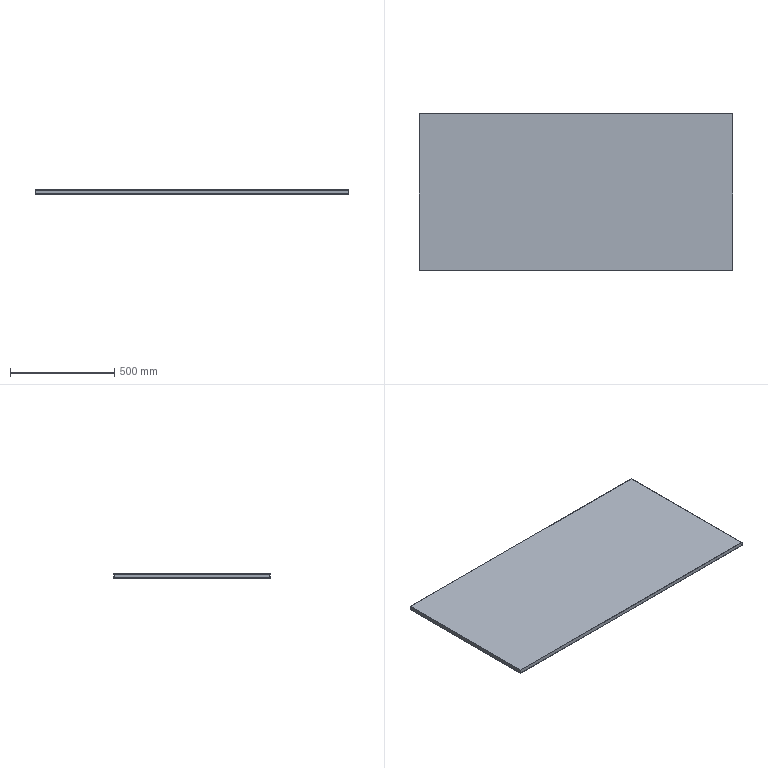Part | STEP file | 1 solid | 16 faces | box 1500 x 750 x 20 mm | volume 1901997 mm3 | plane 16
STEP:
#1=CARTESIAN_POINT('',(0.,0.,0.));
#2=DIRECTION('',(0.,0.,1.));
#3=DIRECTION('',(1.,0.,0.));
#4=AXIS2_PLACEMENT_3D('',#1,#2,#3);
#5=CARTESIAN_POINT('',(750.,-375.,20.));
#6=VERTEX_POINT('',#5);
#7=CARTESIAN_POINT('',(750.,375.,20.));
#8=VERTEX_POINT('',#7);
#9=CARTESIAN_POINT('',(750.,-375.,20.));
#10=DIRECTION('',(0.,1.,0.));
#11=VECTOR('',#10,1.);
#12=LINE('',#9,#11);
#13=CARTESIAN_POINT('',(750.,-375.,20.));
#14=DIRECTION('',(0.,0.,1.));
#15=DIRECTION('',(1.,0.,0.));
#16=AXIS2_PLACEMENT_3D('',#13,#14,#15);
#17=PLANE('',#16);
#18=CARTESIAN_POINT('',(0.,0.));
#19=DIRECTION('',(0.,1.));
#20=VECTOR('',#19,1.);
#21=LINE('',#18,#20);
#22=(GEOMETRIC_REPRESENTATION_CONTEXT(2)PARAMETRIC_REPRESENTATION_CONTEXT()REPRESENTATION_CONTEXT('',''));
#23=DEFINITIONAL_REPRESENTATION('',(#21),#22);
#24=PCURVE('',#17,#23);
#25=CARTESIAN_POINT('',(750.,375.,20.));
#26=DIRECTION('',(-1.,0.,0.));
#27=DIRECTION('',(0.,-1.,0.));
#28=AXIS2_PLACEMENT_3D('',#25,#26,#27);
#29=PLANE('',#28);
#30=CARTESIAN_POINT('',(750.,0.));
#31=DIRECTION('',(-1.,0.));
#32=VECTOR('',#31,1.);
#33=LINE('',#30,#32);
#34=(GEOMETRIC_REPRESENTATION_CONTEXT(2)PARAMETRIC_REPRESENTATION_CONTEXT()REPRESENTATION_CONTEXT('',''));
#35=DEFINITIONAL_REPRESENTATION('',(#33),#34);
#36=PCURVE('',#29,#35);
#37=SURFACE_CURVE('',#12,(#24,#36),.PCURVE_S1.);
#38=EDGE_CURVE('',#6,#8,#37,.T.);
#39=ORIENTED_EDGE('',*,*,#38,.T.);
#40=CARTESIAN_POINT('',(-750.,375.,20.));
#41=VERTEX_POINT('',#40);
#42=CARTESIAN_POINT('',(750.,375.,20.));
#43=DIRECTION('',(-1.,0.,0.));
#44=VECTOR('',#43,1.);
#45=LINE('',#42,#44);
#46=CARTESIAN_POINT('',(0.,750.));
#47=DIRECTION('',(-1.,0.));
#48=VECTOR('',#47,1.);
#49=LINE('',#46,#48);
#50=(GEOMETRIC_REPRESENTATION_CONTEXT(2)PARAMETRIC_REPRESENTATION_CONTEXT()REPRESENTATION_CONTEXT('',''));
#51=DEFINITIONAL_REPRESENTATION('',(#49),#50);
#52=PCURVE('',#17,#51);
#53=CARTESIAN_POINT('',(-750.,375.,20.));
#54=DIRECTION('',(0.,-1.,0.));
#55=DIRECTION('',(0.,0.,-1.));
#56=AXIS2_PLACEMENT_3D('',#53,#54,#55);
#57=PLANE('',#56);
#58=CARTESIAN_POINT('',(0.,1500.));
#59=DIRECTION('',(0.,-1.));
#60=VECTOR('',#59,1.);
#61=LINE('',#58,#60);
#62=(GEOMETRIC_REPRESENTATION_CONTEXT(2)PARAMETRIC_REPRESENTATION_CONTEXT()REPRESENTATION_CONTEXT('',''));
#63=DEFINITIONAL_REPRESENTATION('',(#61),#62);
#64=PCURVE('',#57,#63);
#65=SURFACE_CURVE('',#45,(#52,#64),.PCURVE_S1.);
#66=EDGE_CURVE('',#8,#41,#65,.T.);
#67=ORIENTED_EDGE('',*,*,#66,.T.);
#68=CARTESIAN_POINT('',(-750.,-375.,20.));
#69=VERTEX_POINT('',#68);
#70=CARTESIAN_POINT('',(-750.,-375.,20.));
#71=DIRECTION('',(0.,-1.,0.));
#72=VECTOR('',#71,1.);
#73=LINE('',#70,#72);
#74=CARTESIAN_POINT('',(-1500.,0.));
#75=DIRECTION('',(0.,-1.));
#76=VECTOR('',#75,1.);
#77=LINE('',#74,#76);
#78=(GEOMETRIC_REPRESENTATION_CONTEXT(2)PARAMETRIC_REPRESENTATION_CONTEXT()REPRESENTATION_CONTEXT('',''));
#79=DEFINITIONAL_REPRESENTATION('',(#77),#78);
#80=PCURVE('',#17,#79);
#81=CARTESIAN_POINT('',(-750.,375.,20.));
#82=DIRECTION('',(1.,0.,0.));
#83=DIRECTION('',(0.,1.,0.));
#84=AXIS2_PLACEMENT_3D('',#81,#82,#83);
#85=PLANE('',#84);
#86=CARTESIAN_POINT('',(-750.,0.));
#87=DIRECTION('',(-1.,0.));
#88=VECTOR('',#87,1.);
#89=LINE('',#86,#88);
#90=(GEOMETRIC_REPRESENTATION_CONTEXT(2)PARAMETRIC_REPRESENTATION_CONTEXT()REPRESENTATION_CONTEXT('',''));
#91=DEFINITIONAL_REPRESENTATION('',(#89),#90);
#92=PCURVE('',#85,#91);
#93=SURFACE_CURVE('',#73,(#80,#92),.PCURVE_S1.);
#94=EDGE_CURVE('',#41,#69,#93,.T.);
#95=ORIENTED_EDGE('',*,*,#94,.T.);
#96=CARTESIAN_POINT('',(750.,-375.,20.));
#97=DIRECTION('',(1.,0.,0.));
#98=VECTOR('',#97,1.);
#99=LINE('',#96,#98);
#100=CARTESIAN_POINT('',(0.,0.));
#101=DIRECTION('',(1.,0.));
#102=VECTOR('',#101,1.);
#103=LINE('',#100,#102);
#104=(GEOMETRIC_REPRESENTATION_CONTEXT(2)PARAMETRIC_REPRESENTATION_CONTEXT()REPRESENTATION_CONTEXT('',''));
#105=DEFINITIONAL_REPRESENTATION('',(#103),#104);
#106=PCURVE('',#17,#105);
#107=CARTESIAN_POINT('',(-750.,-375.,20.));
#108=DIRECTION('',(0.,1.,0.));
#109=DIRECTION('',(0.,0.,1.));
#110=AXIS2_PLACEMENT_3D('',#107,#108,#109);
#111=PLANE('',#110);
#112=CARTESIAN_POINT('',(0.,1500.));
#113=DIRECTION('',(0.,1.));
#114=VECTOR('',#113,1.);
#115=LINE('',#112,#114);
#116=(GEOMETRIC_REPRESENTATION_CONTEXT(2)PARAMETRIC_REPRESENTATION_CONTEXT()REPRESENTATION_CONTEXT('',''));
#117=DEFINITIONAL_REPRESENTATION('',(#115),#116);
#118=PCURVE('',#111,#117);
#119=SURFACE_CURVE('',#99,(#106,#118),.PCURVE_S1.);
#120=EDGE_CURVE('',#69,#6,#119,.T.);
#121=ORIENTED_EDGE('',*,*,#120,.T.);
#122=EDGE_LOOP('',(#39,#67,#95,#121));
#123=FACE_BOUND('',#122,.T.);
#124=ADVANCED_FACE('',(#123),#17,.T.);
#125=ORIENTED_EDGE('',*,*,#66,.F.);
#126=CARTESIAN_POINT('',(750.,375.,0.));
#127=VERTEX_POINT('',#126);
#128=CARTESIAN_POINT('',(750.,375.,20.));
#129=DIRECTION('',(0.,0.,1.));
#130=VECTOR('',#129,1.);
#131=LINE('',#128,#130);
#132=CARTESIAN_POINT('',(0.,1500.));
#133=DIRECTION('',(-1.,0.));
#134=VECTOR('',#133,1.);
#135=LINE('',#132,#134);
#136=(GEOMETRIC_REPRESENTATION_CONTEXT(2)PARAMETRIC_REPRESENTATION_CONTEXT()REPRESENTATION_CONTEXT('',''));
#137=DEFINITIONAL_REPRESENTATION('',(#135),#136);
#138=PCURVE('',#57,#137);
#139=CARTESIAN_POINT('',(0.,0.));
#140=DIRECTION('',(0.,1.));
#141=VECTOR('',#140,1.);
#142=LINE('',#139,#141);
#143=(GEOMETRIC_REPRESENTATION_CONTEXT(2)PARAMETRIC_REPRESENTATION_CONTEXT()REPRESENTATION_CONTEXT('',''));
#144=DEFINITIONAL_REPRESENTATION('',(#142),#143);
#145=PCURVE('',#29,#144);
#146=SURFACE_CURVE('',#131,(#138,#145),.PCURVE_S1.);
#147=EDGE_CURVE('',#127,#8,#146,.T.);
#148=ORIENTED_EDGE('',*,*,#147,.F.);
#149=CARTESIAN_POINT('',(-750.,375.,0.));
#150=VERTEX_POINT('',#149);
#151=CARTESIAN_POINT('',(-750.,375.,0.));
#152=DIRECTION('',(1.,0.,0.));
#153=VECTOR('',#152,1.);
#154=LINE('',#151,#153);
#155=CARTESIAN_POINT('',(20.,0.));
#156=DIRECTION('',(0.,1.));
#157=VECTOR('',#156,1.);
#158=LINE('',#155,#157);
#159=(GEOMETRIC_REPRESENTATION_CONTEXT(2)PARAMETRIC_REPRESENTATION_CONTEXT()REPRESENTATION_CONTEXT('',''));
#160=DEFINITIONAL_REPRESENTATION('',(#158),#159);
#161=PCURVE('',#57,#160);
#162=CARTESIAN_POINT('',(750.,-375.,0.));
#163=DIRECTION('',(0.,0.,1.));
#164=DIRECTION('',(1.,0.,0.));
#165=AXIS2_PLACEMENT_3D('',#162,#163,#164);
#166=PLANE('',#165);
#167=CARTESIAN_POINT('',(-1500.,750.));
#168=DIRECTION('',(1.,0.));
#169=VECTOR('',#168,1.);
#170=LINE('',#167,#169);
#171=(GEOMETRIC_REPRESENTATION_CONTEXT(2)PARAMETRIC_REPRESENTATION_CONTEXT()REPRESENTATION_CONTEXT('',''));
#172=DEFINITIONAL_REPRESENTATION('',(#170),#171);
#173=PCURVE('',#166,#172);
#174=SURFACE_CURVE('',#154,(#161,#173),.PCURVE_S1.);
#175=EDGE_CURVE('',#150,#127,#174,.T.);
#176=ORIENTED_EDGE('',*,*,#175,.F.);
#177=CARTESIAN_POINT('',(-750.,375.,20.));
#178=DIRECTION('',(0.,0.,-1.));
#179=VECTOR('',#178,1.);
#180=LINE('',#177,#179);
#181=CARTESIAN_POINT('',(0.,0.));
#182=DIRECTION('',(1.,0.));
#183=VECTOR('',#182,1.);
#184=LINE('',#181,#183);
#185=(GEOMETRIC_REPRESENTATION_CONTEXT(2)PARAMETRIC_REPRESENTATION_CONTEXT()REPRESENTATION_CONTEXT('',''));
#186=DEFINITIONAL_REPRESENTATION('',(#184),#185);
#187=PCURVE('',#57,#186);
#188=CARTESIAN_POINT('',(0.,0.));
#189=DIRECTION('',(0.,-1.));
#190=VECTOR('',#189,1.);
#191=LINE('',#188,#190);
#192=(GEOMETRIC_REPRESENTATION_CONTEXT(2)PARAMETRIC_REPRESENTATION_CONTEXT()REPRESENTATION_CONTEXT('',''));
#193=DEFINITIONAL_REPRESENTATION('',(#191),#192);
#194=PCURVE('',#85,#193);
#195=SURFACE_CURVE('',#180,(#187,#194),.PCURVE_S1.);
#196=EDGE_CURVE('',#41,#150,#195,.T.);
#197=ORIENTED_EDGE('',*,*,#196,.F.);
#198=EDGE_LOOP('',(#125,#148,#176,#197));
#199=FACE_BOUND('',#198,.T.);
#200=ADVANCED_FACE('',(#199),#57,.F.);
#201=ORIENTED_EDGE('',*,*,#38,.F.);
#202=CARTESIAN_POINT('',(750.,-375.,0.));
#203=VERTEX_POINT('',#202);
#204=CARTESIAN_POINT('',(750.,-375.,20.));
#205=DIRECTION('',(0.,0.,1.));
#206=VECTOR('',#205,1.);
#207=LINE('',#204,#206);
#208=CARTESIAN_POINT('',(750.,0.));
#209=DIRECTION('',(0.,1.));
#210=VECTOR('',#209,1.);
#211=LINE('',#208,#210);
#212=(GEOMETRIC_REPRESENTATION_CONTEXT(2)PARAMETRIC_REPRESENTATION_CONTEXT()REPRESENTATION_CONTEXT('',''));
#213=DEFINITIONAL_REPRESENTATION('',(#211),#212);
#214=PCURVE('',#29,#213);
#215=CARTESIAN_POINT('',(0.,1500.));
#216=DIRECTION('',(1.,0.));
#217=VECTOR('',#216,1.);
#218=LINE('',#215,#217);
#219=(GEOMETRIC_REPRESENTATION_CONTEXT(2)PARAMETRIC_REPRESENTATION_CONTEXT()REPRESENTATION_CONTEXT('',''));
#220=DEFINITIONAL_REPRESENTATION('',(#218),#219);
#221=PCURVE('',#111,#220);
#222=SURFACE_CURVE('',#207,(#214,#221),.PCURVE_S1.);
#223=EDGE_CURVE('',#203,#6,#222,.T.);
#224=ORIENTED_EDGE('',*,*,#223,.F.);
#225=CARTESIAN_POINT('',(750.,375.,0.));
#226=DIRECTION('',(0.,-1.,0.));
#227=VECTOR('',#226,1.);
#228=LINE('',#225,#227);
#229=CARTESIAN_POINT('',(0.,-20.));
#230=DIRECTION('',(1.,0.));
#231=VECTOR('',#230,1.);
#232=LINE('',#229,#231);
#233=(GEOMETRIC_REPRESENTATION_CONTEXT(2)PARAMETRIC_REPRESENTATION_CONTEXT()REPRESENTATION_CONTEXT('',''));
#234=DEFINITIONAL_REPRESENTATION('',(#232),#233);
#235=PCURVE('',#29,#234);
#236=CARTESIAN_POINT('',(0.,750.));
#237=DIRECTION('',(0.,-1.));
#238=VECTOR('',#237,1.);
#239=LINE('',#236,#238);
#240=(GEOMETRIC_REPRESENTATION_CONTEXT(2)PARAMETRIC_REPRESENTATION_CONTEXT()REPRESENTATION_CONTEXT('',''));
#241=DEFINITIONAL_REPRESENTATION('',(#239),#240);
#242=PCURVE('',#166,#241);
#243=SURFACE_CURVE('',#228,(#235,#242),.PCURVE_S1.);
#244=EDGE_CURVE('',#127,#203,#243,.T.);
#245=ORIENTED_EDGE('',*,*,#244,.F.);
#246=ORIENTED_EDGE('',*,*,#147,.T.);
#247=EDGE_LOOP('',(#201,#224,#245,#246));
#248=FACE_BOUND('',#247,.T.);
#249=ADVANCED_FACE('',(#248),#29,.F.);
#250=ORIENTED_EDGE('',*,*,#120,.F.);
#251=CARTESIAN_POINT('',(-750.,-375.,0.));
#252=VERTEX_POINT('',#251);
#253=CARTESIAN_POINT('',(-750.,-375.,20.));
#254=DIRECTION('',(0.,0.,1.));
#255=VECTOR('',#254,1.);
#256=LINE('',#253,#255);
#257=CARTESIAN_POINT('',(0.,0.));
#258=DIRECTION('',(1.,0.));
#259=VECTOR('',#258,1.);
#260=LINE('',#257,#259);
#261=(GEOMETRIC_REPRESENTATION_CONTEXT(2)PARAMETRIC_REPRESENTATION_CONTEXT()REPRESENTATION_CONTEXT('',''));
#262=DEFINITIONAL_REPRESENTATION('',(#260),#261);
#263=PCURVE('',#111,#262);
#264=CARTESIAN_POINT('',(-750.,0.));
#265=DIRECTION('',(0.,1.));
#266=VECTOR('',#265,1.);
#267=LINE('',#264,#266);
#268=(GEOMETRIC_REPRESENTATION_CONTEXT(2)PARAMETRIC_REPRESENTATION_CONTEXT()REPRESENTATION_CONTEXT('',''));
#269=DEFINITIONAL_REPRESENTATION('',(#267),#268);
#270=PCURVE('',#85,#269);
#271=SURFACE_CURVE('',#256,(#263,#270),.PCURVE_S1.);
#272=EDGE_CURVE('',#252,#69,#271,.T.);
#273=ORIENTED_EDGE('',*,*,#272,.F.);
#274=CARTESIAN_POINT('',(-750.,-375.,0.));
#275=DIRECTION('',(-1.,0.,0.));
#276=VECTOR('',#275,1.);
#277=LINE('',#274,#276);
#278=CARTESIAN_POINT('',(-20.,0.));
#279=DIRECTION('',(0.,-1.));
#280=VECTOR('',#279,1.);
#281=LINE('',#278,#280);
#282=(GEOMETRIC_REPRESENTATION_CONTEXT(2)PARAMETRIC_REPRESENTATION_CONTEXT()REPRESENTATION_CONTEXT('',''));
#283=DEFINITIONAL_REPRESENTATION('',(#281),#282);
#284=PCURVE('',#111,#283);
#285=CARTESIAN_POINT('',(-1500.,0.));
#286=DIRECTION('',(-1.,0.));
#287=VECTOR('',#286,1.);
#288=LINE('',#285,#287);
#289=(GEOMETRIC_REPRESENTATION_CONTEXT(2)PARAMETRIC_REPRESENTATION_CONTEXT()REPRESENTATION_CONTEXT('',''));
#290=DEFINITIONAL_REPRESENTATION('',(#288),#289);
#291=PCURVE('',#166,#290);
#292=SURFACE_CURVE('',#277,(#284,#291),.PCURVE_S1.);
#293=EDGE_CURVE('',#203,#252,#292,.T.);
#294=ORIENTED_EDGE('',*,*,#293,.F.);
#295=ORIENTED_EDGE('',*,*,#223,.T.);
#296=EDGE_LOOP('',(#250,#273,#294,#295));
#297=FACE_BOUND('',#296,.T.);
#298=ADVANCED_FACE('',(#297),#111,.F.);
#299=ORIENTED_EDGE('',*,*,#94,.F.);
#300=ORIENTED_EDGE('',*,*,#196,.T.);
#301=CARTESIAN_POINT('',(-750.,375.,0.));
#302=DIRECTION('',(0.,1.,0.));
#303=VECTOR('',#302,1.);
#304=LINE('',#301,#303);
#305=CARTESIAN_POINT('',(0.,-20.));
#306=DIRECTION('',(1.,0.));
#307=VECTOR('',#306,1.);
#308=LINE('',#305,#307);
#309=(GEOMETRIC_REPRESENTATION_CONTEXT(2)PARAMETRIC_REPRESENTATION_CONTEXT()REPRESENTATION_CONTEXT('',''));
#310=DEFINITIONAL_REPRESENTATION('',(#308),#309);
#311=PCURVE('',#85,#310);
#312=CARTESIAN_POINT('',(-1500.,750.));
#313=DIRECTION('',(0.,1.));
#314=VECTOR('',#313,1.);
#315=LINE('',#312,#314);
#316=(GEOMETRIC_REPRESENTATION_CONTEXT(2)PARAMETRIC_REPRESENTATION_CONTEXT()REPRESENTATION_CONTEXT('',''));
#317=DEFINITIONAL_REPRESENTATION('',(#315),#316);
#318=PCURVE('',#166,#317);
#319=SURFACE_CURVE('',#304,(#311,#318),.PCURVE_S1.);
#320=EDGE_CURVE('',#252,#150,#319,.T.);
#321=ORIENTED_EDGE('',*,*,#320,.F.);
#322=ORIENTED_EDGE('',*,*,#272,.T.);
#323=EDGE_LOOP('',(#299,#300,#321,#322));
#324=FACE_BOUND('',#323,.T.);
#325=ADVANCED_FACE('',(#324),#85,.F.);
#326=CARTESIAN_POINT('',(735.,360.,0.));
#327=VERTEX_POINT('',#326);
#328=CARTESIAN_POINT('',(735.,-360.,0.));
#329=VERTEX_POINT('',#328);
#330=CARTESIAN_POINT('',(735.,-375.,0.));
#331=DIRECTION('',(0.,-1.,0.));
#332=VECTOR('',#331,1.);
#333=LINE('',#330,#332);
#334=CARTESIAN_POINT('',(-15.,0.));
#335=DIRECTION('',(0.,-1.));
#336=VECTOR('',#335,1.);
#337=LINE('',#334,#336);
#338=(GEOMETRIC_REPRESENTATION_CONTEXT(2)PARAMETRIC_REPRESENTATION_CONTEXT()REPRESENTATION_CONTEXT('',''));
#339=DEFINITIONAL_REPRESENTATION('',(#337),#338);
#340=PCURVE('',#166,#339);
#341=CARTESIAN_POINT('',(735.,360.,1.5));
#342=DIRECTION('',(1.,0.,0.));
#343=DIRECTION('',(0.,0.,-1.));
#344=AXIS2_PLACEMENT_3D('',#341,#342,#343);
#345=PLANE('',#344);
#346=CARTESIAN_POINT('',(1.5,-735.));
#347=DIRECTION('',(0.,-1.));
#348=VECTOR('',#347,1.);
#349=LINE('',#346,#348);
#350=(GEOMETRIC_REPRESENTATION_CONTEXT(2)PARAMETRIC_REPRESENTATION_CONTEXT()REPRESENTATION_CONTEXT('',''));
#351=DEFINITIONAL_REPRESENTATION('',(#349),#350);
#352=PCURVE('',#345,#351);
#353=SURFACE_CURVE('',#333,(#340,#352),.PCURVE_S1.);
#354=EDGE_CURVE('',#327,#329,#353,.T.);
#355=ORIENTED_EDGE('',*,*,#354,.F.);
#356=CARTESIAN_POINT('',(-735.,360.,0.));
#357=VERTEX_POINT('',#356);
#358=CARTESIAN_POINT('',(750.,360.,0.));
#359=DIRECTION('',(1.,0.,0.));
#360=VECTOR('',#359,1.);
#361=LINE('',#358,#360);
#362=CARTESIAN_POINT('',(0.,735.));
#363=DIRECTION('',(1.,0.));
#364=VECTOR('',#363,1.);
#365=LINE('',#362,#364);
#366=(GEOMETRIC_REPRESENTATION_CONTEXT(2)PARAMETRIC_REPRESENTATION_CONTEXT()REPRESENTATION_CONTEXT('',''));
#367=DEFINITIONAL_REPRESENTATION('',(#365),#366);
#368=PCURVE('',#166,#367);
#369=CARTESIAN_POINT('',(735.,360.,1.5));
#370=DIRECTION('',(0.,1.,0.));
#371=DIRECTION('',(0.,0.,1.));
#372=AXIS2_PLACEMENT_3D('',#369,#370,#371);
#373=PLANE('',#372);
#374=CARTESIAN_POINT('',(-1.5,15.));
#375=DIRECTION('',(0.,1.));
#376=VECTOR('',#375,1.);
#377=LINE('',#374,#376);
#378=(GEOMETRIC_REPRESENTATION_CONTEXT(2)PARAMETRIC_REPRESENTATION_CONTEXT()REPRESENTATION_CONTEXT('',''));
#379=DEFINITIONAL_REPRESENTATION('',(#377),#378);
#380=PCURVE('',#373,#379);
#381=SURFACE_CURVE('',#361,(#368,#380),.PCURVE_S1.);
#382=EDGE_CURVE('',#357,#327,#381,.T.);
#383=ORIENTED_EDGE('',*,*,#382,.F.);
#384=CARTESIAN_POINT('',(-735.,-360.,0.));
#385=VERTEX_POINT('',#384);
#386=CARTESIAN_POINT('',(-735.,-375.,0.));
#387=DIRECTION('',(0.,1.,0.));
#388=VECTOR('',#387,1.);
#389=LINE('',#386,#388);
#390=CARTESIAN_POINT('',(-1485.,0.));
#391=DIRECTION('',(0.,1.));
#392=VECTOR('',#391,1.);
#393=LINE('',#390,#392);
#394=(GEOMETRIC_REPRESENTATION_CONTEXT(2)PARAMETRIC_REPRESENTATION_CONTEXT()REPRESENTATION_CONTEXT('',''));
#395=DEFINITIONAL_REPRESENTATION('',(#393),#394);
#396=PCURVE('',#166,#395);
#397=CARTESIAN_POINT('',(-735.,360.,1.5));
#398=DIRECTION('',(-1.,0.,0.));
#399=DIRECTION('',(0.,0.,1.));
#400=AXIS2_PLACEMENT_3D('',#397,#398,#399);
#401=PLANE('',#400);
#402=CARTESIAN_POINT('',(-1.5,-735.));
#403=DIRECTION('',(0.,1.));
#404=VECTOR('',#403,1.);
#405=LINE('',#402,#404);
#406=(GEOMETRIC_REPRESENTATION_CONTEXT(2)PARAMETRIC_REPRESENTATION_CONTEXT()REPRESENTATION_CONTEXT('',''));
#407=DEFINITIONAL_REPRESENTATION('',(#405),#406);
#408=PCURVE('',#401,#407);
#409=SURFACE_CURVE('',#389,(#396,#408),.PCURVE_S1.);
#410=EDGE_CURVE('',#385,#357,#409,.T.);
#411=ORIENTED_EDGE('',*,*,#410,.F.);
#412=CARTESIAN_POINT('',(750.,-360.,0.));
#413=DIRECTION('',(-1.,0.,0.));
#414=VECTOR('',#413,1.);
#415=LINE('',#412,#414);
#416=CARTESIAN_POINT('',(0.,15.));
#417=DIRECTION('',(-1.,0.));
#418=VECTOR('',#417,1.);
#419=LINE('',#416,#418);
#420=(GEOMETRIC_REPRESENTATION_CONTEXT(2)PARAMETRIC_REPRESENTATION_CONTEXT()REPRESENTATION_CONTEXT('',''));
#421=DEFINITIONAL_REPRESENTATION('',(#419),#420);
#422=PCURVE('',#166,#421);
#423=CARTESIAN_POINT('',(735.,-360.,1.5));
#424=DIRECTION('',(0.,-1.,0.));
#425=DIRECTION('',(0.,0.,-1.));
#426=AXIS2_PLACEMENT_3D('',#423,#424,#425);
#427=PLANE('',#426);
#428=CARTESIAN_POINT('',(1.5,15.));
#429=DIRECTION('',(0.,-1.));
#430=VECTOR('',#429,1.);
#431=LINE('',#428,#430);
#432=(GEOMETRIC_REPRESENTATION_CONTEXT(2)PARAMETRIC_REPRESENTATION_CONTEXT()REPRESENTATION_CONTEXT('',''));
#433=DEFINITIONAL_REPRESENTATION('',(#431),#432);
#434=PCURVE('',#427,#433);
#435=SURFACE_CURVE('',#415,(#422,#434),.PCURVE_S1.);
#436=EDGE_CURVE('',#329,#385,#435,.T.);
#437=ORIENTED_EDGE('',*,*,#436,.F.);
#438=EDGE_LOOP('',(#355,#383,#411,#437));
#439=FACE_BOUND('',#438,.T.);
#440=ORIENTED_EDGE('',*,*,#320,.T.);
#441=ORIENTED_EDGE('',*,*,#175,.T.);
#442=ORIENTED_EDGE('',*,*,#244,.T.);
#443=ORIENTED_EDGE('',*,*,#293,.T.);
#444=EDGE_LOOP('',(#440,#441,#442,#443));
#445=FACE_BOUND('',#444,.T.);
#446=ADVANCED_FACE('',(#439,#445),#166,.F.);
#447=CARTESIAN_POINT('',(735.,-360.,1.5));
#448=VERTEX_POINT('',#447);
#449=CARTESIAN_POINT('',(-735.,-360.,1.5));
#450=VERTEX_POINT('',#449);
#451=CARTESIAN_POINT('',(735.,-360.,1.5));
#452=DIRECTION('',(-1.,0.,0.));
#453=VECTOR('',#452,1.);
#454=LINE('',#451,#453);
#455=CARTESIAN_POINT('',(0.,0.));
#456=DIRECTION('',(0.,-1.));
#457=VECTOR('',#456,1.);
#458=LINE('',#455,#457);
#459=(GEOMETRIC_REPRESENTATION_CONTEXT(2)PARAMETRIC_REPRESENTATION_CONTEXT()REPRESENTATION_CONTEXT('',''));
#460=DEFINITIONAL_REPRESENTATION('',(#458),#459);
#461=PCURVE('',#427,#460);
#462=CARTESIAN_POINT('',(-750.,-375.,1.5));
#463=DIRECTION('',(0.,0.,-1.));
#464=DIRECTION('',(-1.,0.,0.));
#465=AXIS2_PLACEMENT_3D('',#462,#463,#464);
#466=PLANE('',#465);
#467=CARTESIAN_POINT('',(-1485.,15.));
#468=DIRECTION('',(1.,0.));
#469=VECTOR('',#468,1.);
#470=LINE('',#467,#469);
#471=(GEOMETRIC_REPRESENTATION_CONTEXT(2)PARAMETRIC_REPRESENTATION_CONTEXT()REPRESENTATION_CONTEXT('',''));
#472=DEFINITIONAL_REPRESENTATION('',(#470),#471);
#473=PCURVE('',#466,#472);
#474=SURFACE_CURVE('',#454,(#461,#473),.PCURVE_S1.);
#475=EDGE_CURVE('',#448,#450,#474,.T.);
#476=ORIENTED_EDGE('',*,*,#475,.F.);
#477=CARTESIAN_POINT('',(735.,-360.,1.5));
#478=DIRECTION('',(0.,0.,1.));
#479=VECTOR('',#478,1.);
#480=LINE('',#477,#479);
#481=CARTESIAN_POINT('',(0.,0.));
#482=DIRECTION('',(-1.,0.));
#483=VECTOR('',#482,1.);
#484=LINE('',#481,#483);
#485=(GEOMETRIC_REPRESENTATION_CONTEXT(2)PARAMETRIC_REPRESENTATION_CONTEXT()REPRESENTATION_CONTEXT('',''));
#486=DEFINITIONAL_REPRESENTATION('',(#484),#485);
#487=PCURVE('',#427,#486);
#488=CARTESIAN_POINT('',(0.,-720.));
#489=DIRECTION('',(-1.,0.));
#490=VECTOR('',#489,1.);
#491=LINE('',#488,#490);
#492=(GEOMETRIC_REPRESENTATION_CONTEXT(2)PARAMETRIC_REPRESENTATION_CONTEXT()REPRESENTATION_CONTEXT('',''));
#493=DEFINITIONAL_REPRESENTATION('',(#491),#492);
#494=PCURVE('',#345,#493);
#495=SURFACE_CURVE('',#480,(#487,#494),.PCURVE_S1.);
#496=EDGE_CURVE('',#329,#448,#495,.T.);
#497=ORIENTED_EDGE('',*,*,#496,.F.);
#498=ORIENTED_EDGE('',*,*,#436,.T.);
#499=CARTESIAN_POINT('',(-735.,-360.,1.5));
#500=DIRECTION('',(0.,0.,-1.));
#501=VECTOR('',#500,1.);
#502=LINE('',#499,#501);
#503=CARTESIAN_POINT('',(0.,-1470.));
#504=DIRECTION('',(1.,0.));
#505=VECTOR('',#504,1.);
#506=LINE('',#503,#505);
#507=(GEOMETRIC_REPRESENTATION_CONTEXT(2)PARAMETRIC_REPRESENTATION_CONTEXT()REPRESENTATION_CONTEXT('',''));
#508=DEFINITIONAL_REPRESENTATION('',(#506),#507);
#509=PCURVE('',#427,#508);
#510=CARTESIAN_POINT('',(0.,-720.));
#511=DIRECTION('',(-1.,0.));
#512=VECTOR('',#511,1.);
#513=LINE('',#510,#512);
#514=(GEOMETRIC_REPRESENTATION_CONTEXT(2)PARAMETRIC_REPRESENTATION_CONTEXT()REPRESENTATION_CONTEXT('',''));
#515=DEFINITIONAL_REPRESENTATION('',(#513),#514);
#516=PCURVE('',#401,#515);
#517=SURFACE_CURVE('',#502,(#509,#516),.PCURVE_S1.);
#518=EDGE_CURVE('',#450,#385,#517,.T.);
#519=ORIENTED_EDGE('',*,*,#518,.F.);
#520=EDGE_LOOP('',(#476,#497,#498,#519));
#521=FACE_BOUND('',#520,.T.);
#522=ADVANCED_FACE('',(#521),#427,.F.);
#523=CARTESIAN_POINT('',(735.,360.,1.5));
#524=VERTEX_POINT('',#523);
#525=CARTESIAN_POINT('',(735.,360.,1.5));
#526=DIRECTION('',(0.,-1.,0.));
#527=VECTOR('',#526,1.);
#528=LINE('',#525,#527);
#529=CARTESIAN_POINT('',(0.,0.));
#530=DIRECTION('',(0.,-1.));
#531=VECTOR('',#530,1.);
#532=LINE('',#529,#531);
#533=(GEOMETRIC_REPRESENTATION_CONTEXT(2)PARAMETRIC_REPRESENTATION_CONTEXT()REPRESENTATION_CONTEXT('',''));
#534=DEFINITIONAL_REPRESENTATION('',(#532),#533);
#535=PCURVE('',#345,#534);
#536=CARTESIAN_POINT('',(-1485.,735.));
#537=DIRECTION('',(0.,-1.));
#538=VECTOR('',#537,1.);
#539=LINE('',#536,#538);
#540=(GEOMETRIC_REPRESENTATION_CONTEXT(2)PARAMETRIC_REPRESENTATION_CONTEXT()REPRESENTATION_CONTEXT('',''));
#541=DEFINITIONAL_REPRESENTATION('',(#539),#540);
#542=PCURVE('',#466,#541);
#543=SURFACE_CURVE('',#528,(#535,#542),.PCURVE_S1.);
#544=EDGE_CURVE('',#524,#448,#543,.T.);
#545=ORIENTED_EDGE('',*,*,#544,.F.);
#546=CARTESIAN_POINT('',(735.,360.,1.5));
#547=DIRECTION('',(0.,0.,1.));
#548=VECTOR('',#547,1.);
#549=LINE('',#546,#548);
#550=CARTESIAN_POINT('',(0.,0.));
#551=DIRECTION('',(-1.,0.));
#552=VECTOR('',#551,1.);
#553=LINE('',#550,#552);
#554=(GEOMETRIC_REPRESENTATION_CONTEXT(2)PARAMETRIC_REPRESENTATION_CONTEXT()REPRESENTATION_CONTEXT('',''));
#555=DEFINITIONAL_REPRESENTATION('',(#553),#554);
#556=PCURVE('',#345,#555);
#557=CARTESIAN_POINT('',(0.,0.));
#558=DIRECTION('',(1.,0.));
#559=VECTOR('',#558,1.);
#560=LINE('',#557,#559);
#561=(GEOMETRIC_REPRESENTATION_CONTEXT(2)PARAMETRIC_REPRESENTATION_CONTEXT()REPRESENTATION_CONTEXT('',''));
#562=DEFINITIONAL_REPRESENTATION('',(#560),#561);
#563=PCURVE('',#373,#562);
#564=SURFACE_CURVE('',#549,(#556,#563),.PCURVE_S1.);
#565=EDGE_CURVE('',#327,#524,#564,.T.);
#566=ORIENTED_EDGE('',*,*,#565,.F.);
#567=ORIENTED_EDGE('',*,*,#354,.T.);
#568=ORIENTED_EDGE('',*,*,#496,.T.);
#569=EDGE_LOOP('',(#545,#566,#567,#568));
#570=FACE_BOUND('',#569,.T.);
#571=ADVANCED_FACE('',(#570),#345,.F.);
#572=CARTESIAN_POINT('',(-735.,360.,1.5));
#573=VERTEX_POINT('',#572);
#574=CARTESIAN_POINT('',(735.,360.,1.5));
#575=DIRECTION('',(1.,0.,0.));
#576=VECTOR('',#575,1.);
#577=LINE('',#574,#576);
#578=CARTESIAN_POINT('',(0.,0.));
#579=DIRECTION('',(0.,1.));
#580=VECTOR('',#579,1.);
#581=LINE('',#578,#580);
#582=(GEOMETRIC_REPRESENTATION_CONTEXT(2)PARAMETRIC_REPRESENTATION_CONTEXT()REPRESENTATION_CONTEXT('',''));
#583=DEFINITIONAL_REPRESENTATION('',(#581),#582);
#584=PCURVE('',#373,#583);
#585=CARTESIAN_POINT('',(-1485.,735.));
#586=DIRECTION('',(-1.,0.));
#587=VECTOR('',#586,1.);
#588=LINE('',#585,#587);
#589=(GEOMETRIC_REPRESENTATION_CONTEXT(2)PARAMETRIC_REPRESENTATION_CONTEXT()REPRESENTATION_CONTEXT('',''));
#590=DEFINITIONAL_REPRESENTATION('',(#588),#589);
#591=PCURVE('',#466,#590);
#592=SURFACE_CURVE('',#577,(#584,#591),.PCURVE_S1.);
#593=EDGE_CURVE('',#573,#524,#592,.T.);
#594=ORIENTED_EDGE('',*,*,#593,.F.);
#595=CARTESIAN_POINT('',(-735.,360.,1.5));
#596=DIRECTION('',(0.,0.,1.));
#597=VECTOR('',#596,1.);
#598=LINE('',#595,#597);
#599=CARTESIAN_POINT('',(0.,-1470.));
#600=DIRECTION('',(1.,0.));
#601=VECTOR('',#600,1.);
#602=LINE('',#599,#601);
#603=(GEOMETRIC_REPRESENTATION_CONTEXT(2)PARAMETRIC_REPRESENTATION_CONTEXT()REPRESENTATION_CONTEXT('',''));
#604=DEFINITIONAL_REPRESENTATION('',(#602),#603);
#605=PCURVE('',#373,#604);
#606=CARTESIAN_POINT('',(0.,0.));
#607=DIRECTION('',(1.,0.));
#608=VECTOR('',#607,1.);
#609=LINE('',#606,#608);
#610=(GEOMETRIC_REPRESENTATION_CONTEXT(2)PARAMETRIC_REPRESENTATION_CONTEXT()REPRESENTATION_CONTEXT('',''));
#611=DEFINITIONAL_REPRESENTATION('',(#609),#610);
#612=PCURVE('',#401,#611);
#613=SURFACE_CURVE('',#598,(#605,#612),.PCURVE_S1.);
#614=EDGE_CURVE('',#357,#573,#613,.T.);
#615=ORIENTED_EDGE('',*,*,#614,.F.);
#616=ORIENTED_EDGE('',*,*,#382,.T.);
#617=ORIENTED_EDGE('',*,*,#565,.T.);
#618=EDGE_LOOP('',(#594,#615,#616,#617));
#619=FACE_BOUND('',#618,.T.);
#620=ADVANCED_FACE('',(#619),#373,.F.);
#621=CARTESIAN_POINT('',(-735.,360.,1.5));
#622=DIRECTION('',(0.,1.,0.));
#623=VECTOR('',#622,1.);
#624=LINE('',#621,#623);
#625=CARTESIAN_POINT('',(0.,0.));
#626=DIRECTION('',(0.,1.));
#627=VECTOR('',#626,1.);
#628=LINE('',#625,#627);
#629=(GEOMETRIC_REPRESENTATION_CONTEXT(2)PARAMETRIC_REPRESENTATION_CONTEXT()REPRESENTATION_CONTEXT('',''));
#630=DEFINITIONAL_REPRESENTATION('',(#628),#629);
#631=PCURVE('',#401,#630);
#632=CARTESIAN_POINT('',(-15.,735.));
#633=DIRECTION('',(0.,1.));
#634=VECTOR('',#633,1.);
#635=LINE('',#632,#634);
#636=(GEOMETRIC_REPRESENTATION_CONTEXT(2)PARAMETRIC_REPRESENTATION_CONTEXT()REPRESENTATION_CONTEXT('',''));
#637=DEFINITIONAL_REPRESENTATION('',(#635),#636);
#638=PCURVE('',#466,#637);
#639=SURFACE_CURVE('',#624,(#631,#638),.PCURVE_S1.);
#640=EDGE_CURVE('',#450,#573,#639,.T.);
#641=ORIENTED_EDGE('',*,*,#640,.F.);
#642=ORIENTED_EDGE('',*,*,#518,.T.);
#643=ORIENTED_EDGE('',*,*,#410,.T.);
#644=ORIENTED_EDGE('',*,*,#614,.T.);
#645=EDGE_LOOP('',(#641,#642,#643,#644));
#646=FACE_BOUND('',#645,.T.);
#647=ADVANCED_FACE('',(#646),#401,.F.);
#648=ORIENTED_EDGE('',*,*,#593,.T.);
#649=ORIENTED_EDGE('',*,*,#544,.T.);
#650=ORIENTED_EDGE('',*,*,#475,.T.);
#651=ORIENTED_EDGE('',*,*,#640,.T.);
#652=EDGE_LOOP('',(#648,#649,#650,#651));
#653=FACE_BOUND('',#652,.T.);
#654=CARTESIAN_POINT('',(-748.5,-373.5,1.5));
#655=VERTEX_POINT('',#654);
#656=CARTESIAN_POINT('',(-748.5,373.5,1.5));
#657=VERTEX_POINT('',#656);
#658=CARTESIAN_POINT('',(-748.5,-375.,1.5));
#659=DIRECTION('',(0.,1.,0.));
#660=VECTOR('',#659,1.);
#661=LINE('',#658,#660);
#662=CARTESIAN_POINT('',(-1.5,0.));
#663=DIRECTION('',(0.,1.));
#664=VECTOR('',#663,1.);
#665=LINE('',#662,#664);
#666=(GEOMETRIC_REPRESENTATION_CONTEXT(2)PARAMETRIC_REPRESENTATION_CONTEXT()REPRESENTATION_CONTEXT('',''));
#667=DEFINITIONAL_REPRESENTATION('',(#665),#666);
#668=PCURVE('',#466,#667);
#669=CARTESIAN_POINT('',(-748.5,375.,20.));
#670=DIRECTION('',(1.,0.,0.));
#671=DIRECTION('',(0.,1.,0.));
#672=AXIS2_PLACEMENT_3D('',#669,#670,#671);
#673=PLANE('',#672);
#674=CARTESIAN_POINT('',(-750.,-18.5));
#675=DIRECTION('',(1.,0.));
#676=VECTOR('',#675,1.);
#677=LINE('',#674,#676);
#678=(GEOMETRIC_REPRESENTATION_CONTEXT(2)PARAMETRIC_REPRESENTATION_CONTEXT()REPRESENTATION_CONTEXT('',''));
#679=DEFINITIONAL_REPRESENTATION('',(#677),#678);
#680=PCURVE('',#673,#679);
#681=SURFACE_CURVE('',#661,(#668,#680),.PCURVE_S1.);
#682=EDGE_CURVE('',#655,#657,#681,.T.);
#683=ORIENTED_EDGE('',*,*,#682,.F.);
#684=CARTESIAN_POINT('',(748.5,-373.5,1.5));
#685=VERTEX_POINT('',#684);
#686=CARTESIAN_POINT('',(-750.,-373.5,1.5));
#687=DIRECTION('',(-1.,0.,0.));
#688=VECTOR('',#687,1.);
#689=LINE('',#686,#688);
#690=CARTESIAN_POINT('',(0.,1.5));
#691=DIRECTION('',(1.,0.));
#692=VECTOR('',#691,1.);
#693=LINE('',#690,#692);
#694=(GEOMETRIC_REPRESENTATION_CONTEXT(2)PARAMETRIC_REPRESENTATION_CONTEXT()REPRESENTATION_CONTEXT('',''));
#695=DEFINITIONAL_REPRESENTATION('',(#693),#694);
#696=PCURVE('',#466,#695);
#697=CARTESIAN_POINT('',(-750.,-373.5,20.));
#698=DIRECTION('',(0.,1.,0.));
#699=DIRECTION('',(0.,0.,1.));
#700=AXIS2_PLACEMENT_3D('',#697,#698,#699);
#701=PLANE('',#700);
#702=CARTESIAN_POINT('',(-18.5,0.));
#703=DIRECTION('',(0.,-1.));
#704=VECTOR('',#703,1.);
#705=LINE('',#702,#704);
#706=(GEOMETRIC_REPRESENTATION_CONTEXT(2)PARAMETRIC_REPRESENTATION_CONTEXT()REPRESENTATION_CONTEXT('',''));
#707=DEFINITIONAL_REPRESENTATION('',(#705),#706);
#708=PCURVE('',#701,#707);
#709=SURFACE_CURVE('',#689,(#696,#708),.PCURVE_S1.);
#710=EDGE_CURVE('',#685,#655,#709,.T.);
#711=ORIENTED_EDGE('',*,*,#710,.F.);
#712=CARTESIAN_POINT('',(748.5,373.5,1.5));
#713=VERTEX_POINT('',#712);
#714=CARTESIAN_POINT('',(748.5,-375.,1.5));
#715=DIRECTION('',(0.,-1.,0.));
#716=VECTOR('',#715,1.);
#717=LINE('',#714,#716);
#718=CARTESIAN_POINT('',(-1498.5,0.));
#719=DIRECTION('',(0.,-1.));
#720=VECTOR('',#719,1.);
#721=LINE('',#718,#720);
#722=(GEOMETRIC_REPRESENTATION_CONTEXT(2)PARAMETRIC_REPRESENTATION_CONTEXT()REPRESENTATION_CONTEXT('',''));
#723=DEFINITIONAL_REPRESENTATION('',(#721),#722);
#724=PCURVE('',#466,#723);
#725=CARTESIAN_POINT('',(748.5,375.,20.));
#726=DIRECTION('',(-1.,0.,0.));
#727=DIRECTION('',(0.,-1.,0.));
#728=AXIS2_PLACEMENT_3D('',#725,#726,#727);
#729=PLANE('',#728);
#730=CARTESIAN_POINT('',(750.,-18.5));
#731=DIRECTION('',(1.,0.));
#732=VECTOR('',#731,1.);
#733=LINE('',#730,#732);
#734=(GEOMETRIC_REPRESENTATION_CONTEXT(2)PARAMETRIC_REPRESENTATION_CONTEXT()REPRESENTATION_CONTEXT('',''));
#735=DEFINITIONAL_REPRESENTATION('',(#733),#734);
#736=PCURVE('',#729,#735);
#737=SURFACE_CURVE('',#717,(#724,#736),.PCURVE_S1.);
#738=EDGE_CURVE('',#713,#685,#737,.T.);
#739=ORIENTED_EDGE('',*,*,#738,.F.);
#740=CARTESIAN_POINT('',(-750.,373.5,1.5));
#741=DIRECTION('',(1.,0.,0.));
#742=VECTOR('',#741,1.);
#743=LINE('',#740,#742);
#744=CARTESIAN_POINT('',(0.,748.5));
#745=DIRECTION('',(-1.,0.));
#746=VECTOR('',#745,1.);
#747=LINE('',#744,#746);
#748=(GEOMETRIC_REPRESENTATION_CONTEXT(2)PARAMETRIC_REPRESENTATION_CONTEXT()REPRESENTATION_CONTEXT('',''));
#749=DEFINITIONAL_REPRESENTATION('',(#747),#748);
#750=PCURVE('',#466,#749);
#751=CARTESIAN_POINT('',(-750.,373.5,20.));
#752=DIRECTION('',(0.,-1.,0.));
#753=DIRECTION('',(0.,0.,-1.));
#754=AXIS2_PLACEMENT_3D('',#751,#752,#753);
#755=PLANE('',#754);
#756=CARTESIAN_POINT('',(18.5,0.));
#757=DIRECTION('',(0.,1.));
#758=VECTOR('',#757,1.);
#759=LINE('',#756,#758);
#760=(GEOMETRIC_REPRESENTATION_CONTEXT(2)PARAMETRIC_REPRESENTATION_CONTEXT()REPRESENTATION_CONTEXT('',''));
#761=DEFINITIONAL_REPRESENTATION('',(#759),#760);
#762=PCURVE('',#755,#761);
#763=SURFACE_CURVE('',#743,(#750,#762),.PCURVE_S1.);
#764=EDGE_CURVE('',#657,#713,#763,.T.);
#765=ORIENTED_EDGE('',*,*,#764,.F.);
#766=EDGE_LOOP('',(#683,#711,#739,#765));
#767=FACE_BOUND('',#766,.T.);
#768=ADVANCED_FACE('',(#653,#767),#466,.F.);
#769=CARTESIAN_POINT('',(-748.5,373.5,18.5));
#770=VERTEX_POINT('',#769);
#771=CARTESIAN_POINT('',(-748.5,373.5,20.));
#772=DIRECTION('',(0.,0.,-1.));
#773=VECTOR('',#772,1.);
#774=LINE('',#771,#773);
#775=CARTESIAN_POINT('',(0.,1.5));
#776=DIRECTION('',(1.,0.));
#777=VECTOR('',#776,1.);
#778=LINE('',#775,#777);
#779=(GEOMETRIC_REPRESENTATION_CONTEXT(2)PARAMETRIC_REPRESENTATION_CONTEXT()REPRESENTATION_CONTEXT('',''));
#780=DEFINITIONAL_REPRESENTATION('',(#778),#779);
#781=PCURVE('',#755,#780);
#782=CARTESIAN_POINT('',(-1.5,0.));
#783=DIRECTION('',(0.,-1.));
#784=VECTOR('',#783,1.);
#785=LINE('',#782,#784);
#786=(GEOMETRIC_REPRESENTATION_CONTEXT(2)PARAMETRIC_REPRESENTATION_CONTEXT()REPRESENTATION_CONTEXT('',''));
#787=DEFINITIONAL_REPRESENTATION('',(#785),#786);
#788=PCURVE('',#673,#787);
#789=SURFACE_CURVE('',#774,(#781,#788),.PCURVE_S1.);
#790=EDGE_CURVE('',#770,#657,#789,.T.);
#791=ORIENTED_EDGE('',*,*,#790,.T.);
#792=ORIENTED_EDGE('',*,*,#764,.T.);
#793=CARTESIAN_POINT('',(748.5,373.5,18.5));
#794=VERTEX_POINT('',#793);
#795=CARTESIAN_POINT('',(748.5,373.5,20.));
#796=DIRECTION('',(0.,0.,1.));
#797=VECTOR('',#796,1.);
#798=LINE('',#795,#797);
#799=CARTESIAN_POINT('',(0.,1498.5));
#800=DIRECTION('',(-1.,0.));
#801=VECTOR('',#800,1.);
#802=LINE('',#799,#801);
#803=(GEOMETRIC_REPRESENTATION_CONTEXT(2)PARAMETRIC_REPRESENTATION_CONTEXT()REPRESENTATION_CONTEXT('',''));
#804=DEFINITIONAL_REPRESENTATION('',(#802),#803);
#805=PCURVE('',#755,#804);
#806=CARTESIAN_POINT('',(1.5,0.));
#807=DIRECTION('',(0.,1.));
#808=VECTOR('',#807,1.);
#809=LINE('',#806,#808);
#810=(GEOMETRIC_REPRESENTATION_CONTEXT(2)PARAMETRIC_REPRESENTATION_CONTEXT()REPRESENTATION_CONTEXT('',''));
#811=DEFINITIONAL_REPRESENTATION('',(#809),#810);
#812=PCURVE('',#729,#811);
#813=SURFACE_CURVE('',#798,(#805,#812),.PCURVE_S1.);
#814=EDGE_CURVE('',#713,#794,#813,.T.);
#815=ORIENTED_EDGE('',*,*,#814,.T.);
#816=CARTESIAN_POINT('',(-750.,373.5,18.5));
#817=DIRECTION('',(-1.,0.,0.));
#818=VECTOR('',#817,1.);
#819=LINE('',#816,#818);
#820=CARTESIAN_POINT('',(1.5,0.));
#821=DIRECTION('',(0.,-1.));
#822=VECTOR('',#821,1.);
#823=LINE('',#820,#822);
#824=(GEOMETRIC_REPRESENTATION_CONTEXT(2)PARAMETRIC_REPRESENTATION_CONTEXT()REPRESENTATION_CONTEXT('',''));
#825=DEFINITIONAL_REPRESENTATION('',(#823),#824);
#826=PCURVE('',#755,#825);
#827=CARTESIAN_POINT('',(750.,-375.,18.5));
#828=DIRECTION('',(0.,0.,1.));
#829=DIRECTION('',(1.,0.,0.));
#830=AXIS2_PLACEMENT_3D('',#827,#828,#829);
#831=PLANE('',#830);
#832=CARTESIAN_POINT('',(-1500.,748.5));
#833=DIRECTION('',(-1.,0.));
#834=VECTOR('',#833,1.);
#835=LINE('',#832,#834);
#836=(GEOMETRIC_REPRESENTATION_CONTEXT(2)PARAMETRIC_REPRESENTATION_CONTEXT()REPRESENTATION_CONTEXT('',''));
#837=DEFINITIONAL_REPRESENTATION('',(#835),#836);
#838=PCURVE('',#831,#837);
#839=SURFACE_CURVE('',#819,(#826,#838),.PCURVE_S1.);
#840=EDGE_CURVE('',#794,#770,#839,.T.);
#841=ORIENTED_EDGE('',*,*,#840,.T.);
#842=EDGE_LOOP('',(#791,#792,#815,#841));
#843=FACE_BOUND('',#842,.T.);
#844=ADVANCED_FACE('',(#843),#755,.T.);
#845=CARTESIAN_POINT('',(-748.5,-373.5,18.5));
#846=VERTEX_POINT('',#845);
#847=CARTESIAN_POINT('',(-748.5,-373.5,20.));
#848=DIRECTION('',(0.,0.,-1.));
#849=VECTOR('',#848,1.);
#850=LINE('',#847,#849);
#851=CARTESIAN_POINT('',(-748.5,0.));
#852=DIRECTION('',(0.,-1.));
#853=VECTOR('',#852,1.);
#854=LINE('',#851,#853);
#855=(GEOMETRIC_REPRESENTATION_CONTEXT(2)PARAMETRIC_REPRESENTATION_CONTEXT()REPRESENTATION_CONTEXT('',''));
#856=DEFINITIONAL_REPRESENTATION('',(#854),#855);
#857=PCURVE('',#673,#856);
#858=CARTESIAN_POINT('',(0.,1.5));
#859=DIRECTION('',(-1.,0.));
#860=VECTOR('',#859,1.);
#861=LINE('',#858,#860);
#862=(GEOMETRIC_REPRESENTATION_CONTEXT(2)PARAMETRIC_REPRESENTATION_CONTEXT()REPRESENTATION_CONTEXT('',''));
#863=DEFINITIONAL_REPRESENTATION('',(#861),#862);
#864=PCURVE('',#701,#863);
#865=SURFACE_CURVE('',#850,(#857,#864),.PCURVE_S1.);
#866=EDGE_CURVE('',#846,#655,#865,.T.);
#867=ORIENTED_EDGE('',*,*,#866,.T.);
#868=ORIENTED_EDGE('',*,*,#682,.T.);
#869=ORIENTED_EDGE('',*,*,#790,.F.);
#870=CARTESIAN_POINT('',(-748.5,375.,18.5));
#871=DIRECTION('',(0.,-1.,0.));
#872=VECTOR('',#871,1.);
#873=LINE('',#870,#872);
#874=CARTESIAN_POINT('',(0.,-1.5));
#875=DIRECTION('',(-1.,0.));
#876=VECTOR('',#875,1.);
#877=LINE('',#874,#876);
#878=(GEOMETRIC_REPRESENTATION_CONTEXT(2)PARAMETRIC_REPRESENTATION_CONTEXT()REPRESENTATION_CONTEXT('',''));
#879=DEFINITIONAL_REPRESENTATION('',(#877),#878);
#880=PCURVE('',#673,#879);
#881=CARTESIAN_POINT('',(-1498.5,750.));
#882=DIRECTION('',(0.,-1.));
#883=VECTOR('',#882,1.);
#884=LINE('',#881,#883);
#885=(GEOMETRIC_REPRESENTATION_CONTEXT(2)PARAMETRIC_REPRESENTATION_CONTEXT()REPRESENTATION_CONTEXT('',''));
#886=DEFINITIONAL_REPRESENTATION('',(#884),#885);
#887=PCURVE('',#831,#886);
#888=SURFACE_CURVE('',#873,(#880,#887),.PCURVE_S1.);
#889=EDGE_CURVE('',#770,#846,#888,.T.);
#890=ORIENTED_EDGE('',*,*,#889,.T.);
#891=EDGE_LOOP('',(#867,#868,#869,#890));
#892=FACE_BOUND('',#891,.T.);
#893=ADVANCED_FACE('',(#892),#673,.T.);
#894=CARTESIAN_POINT('',(748.5,-373.5,18.5));
#895=VERTEX_POINT('',#894);
#896=CARTESIAN_POINT('',(748.5,-373.5,20.));
#897=DIRECTION('',(0.,0.,-1.));
#898=VECTOR('',#897,1.);
#899=LINE('',#896,#898);
#900=CARTESIAN_POINT('',(0.,1498.5));
#901=DIRECTION('',(-1.,0.));
#902=VECTOR('',#901,1.);
#903=LINE('',#900,#902);
#904=(GEOMETRIC_REPRESENTATION_CONTEXT(2)PARAMETRIC_REPRESENTATION_CONTEXT()REPRESENTATION_CONTEXT('',''));
#905=DEFINITIONAL_REPRESENTATION('',(#903),#904);
#906=PCURVE('',#701,#905);
#907=CARTESIAN_POINT('',(748.5,0.));
#908=DIRECTION('',(0.,-1.));
#909=VECTOR('',#908,1.);
#910=LINE('',#907,#909);
#911=(GEOMETRIC_REPRESENTATION_CONTEXT(2)PARAMETRIC_REPRESENTATION_CONTEXT()REPRESENTATION_CONTEXT('',''));
#912=DEFINITIONAL_REPRESENTATION('',(#910),#911);
#913=PCURVE('',#729,#912);
#914=SURFACE_CURVE('',#899,(#906,#913),.PCURVE_S1.);
#915=EDGE_CURVE('',#895,#685,#914,.T.);
#916=ORIENTED_EDGE('',*,*,#915,.T.);
#917=ORIENTED_EDGE('',*,*,#710,.T.);
#918=ORIENTED_EDGE('',*,*,#866,.F.);
#919=CARTESIAN_POINT('',(-750.,-373.5,18.5));
#920=DIRECTION('',(1.,0.,0.));
#921=VECTOR('',#920,1.);
#922=LINE('',#919,#921);
#923=CARTESIAN_POINT('',(-1.5,0.));
#924=DIRECTION('',(0.,1.));
#925=VECTOR('',#924,1.);
#926=LINE('',#923,#925);
#927=(GEOMETRIC_REPRESENTATION_CONTEXT(2)PARAMETRIC_REPRESENTATION_CONTEXT()REPRESENTATION_CONTEXT('',''));
#928=DEFINITIONAL_REPRESENTATION('',(#926),#927);
#929=PCURVE('',#701,#928);
#930=CARTESIAN_POINT('',(-1500.,1.5));
#931=DIRECTION('',(1.,0.));
#932=VECTOR('',#931,1.);
#933=LINE('',#930,#932);
#934=(GEOMETRIC_REPRESENTATION_CONTEXT(2)PARAMETRIC_REPRESENTATION_CONTEXT()REPRESENTATION_CONTEXT('',''));
#935=DEFINITIONAL_REPRESENTATION('',(#933),#934);
#936=PCURVE('',#831,#935);
#937=SURFACE_CURVE('',#922,(#929,#936),.PCURVE_S1.);
#938=EDGE_CURVE('',#846,#895,#937,.T.);
#939=ORIENTED_EDGE('',*,*,#938,.T.);
#940=EDGE_LOOP('',(#916,#917,#918,#939));
#941=FACE_BOUND('',#940,.T.);
#942=ADVANCED_FACE('',(#941),#701,.T.);
#943=ORIENTED_EDGE('',*,*,#814,.F.);
#944=ORIENTED_EDGE('',*,*,#738,.T.);
#945=ORIENTED_EDGE('',*,*,#915,.F.);
#946=CARTESIAN_POINT('',(748.5,375.,18.5));
#947=DIRECTION('',(0.,1.,0.));
#948=VECTOR('',#947,1.);
#949=LINE('',#946,#948);
#950=CARTESIAN_POINT('',(0.,-1.5));
#951=DIRECTION('',(-1.,0.));
#952=VECTOR('',#951,1.);
#953=LINE('',#950,#952);
#954=(GEOMETRIC_REPRESENTATION_CONTEXT(2)PARAMETRIC_REPRESENTATION_CONTEXT()REPRESENTATION_CONTEXT('',''));
#955=DEFINITIONAL_REPRESENTATION('',(#953),#954);
#956=PCURVE('',#729,#955);
#957=CARTESIAN_POINT('',(-1.5,750.));
#958=DIRECTION('',(0.,1.));
#959=VECTOR('',#958,1.);
#960=LINE('',#957,#959);
#961=(GEOMETRIC_REPRESENTATION_CONTEXT(2)PARAMETRIC_REPRESENTATION_CONTEXT()REPRESENTATION_CONTEXT('',''));
#962=DEFINITIONAL_REPRESENTATION('',(#960),#961);
#963=PCURVE('',#831,#962);
#964=SURFACE_CURVE('',#949,(#956,#963),.PCURVE_S1.);
#965=EDGE_CURVE('',#895,#794,#964,.T.);
#966=ORIENTED_EDGE('',*,*,#965,.T.);
#967=EDGE_LOOP('',(#943,#944,#945,#966));
#968=FACE_BOUND('',#967,.T.);
#969=ADVANCED_FACE('',(#968),#729,.T.);
#970=ORIENTED_EDGE('',*,*,#889,.F.);
#971=ORIENTED_EDGE('',*,*,#840,.F.);
#972=ORIENTED_EDGE('',*,*,#965,.F.);
#973=ORIENTED_EDGE('',*,*,#938,.F.);
#974=EDGE_LOOP('',(#970,#971,#972,#973));
#975=FACE_BOUND('',#974,.T.);
#976=ADVANCED_FACE('',(#975),#831,.F.);
#977=CLOSED_SHELL('',(#124,#200,#249,#298,#325,#446,#522,#571,#620,#647,#768,#844,#893,#942,#969,#976));
#978=MANIFOLD_SOLID_BREP('',#977);
#979=(LENGTH_UNIT()NAMED_UNIT(*)SI_UNIT(.MILLI.,.METRE.));
#980=UNCERTAINTY_MEASURE_WITH_UNIT(LENGTH_MEASURE(0.0000001),#979,'','');
#981=(NAMED_UNIT(*)PLANE_ANGLE_UNIT()SI_UNIT($,.RADIAN.));
#982=(NAMED_UNIT(*)SI_UNIT($,.STERADIAN.)SOLID_ANGLE_UNIT());
#983=(GEOMETRIC_REPRESENTATION_CONTEXT(3)GLOBAL_UNCERTAINTY_ASSIGNED_CONTEXT((#980))GLOBAL_UNIT_ASSIGNED_CONTEXT((#979,#981,#982))REPRESENTATION_CONTEXT('',''));
#984=ADVANCED_BREP_SHAPE_REPRESENTATION('',(#4,#978),#983);